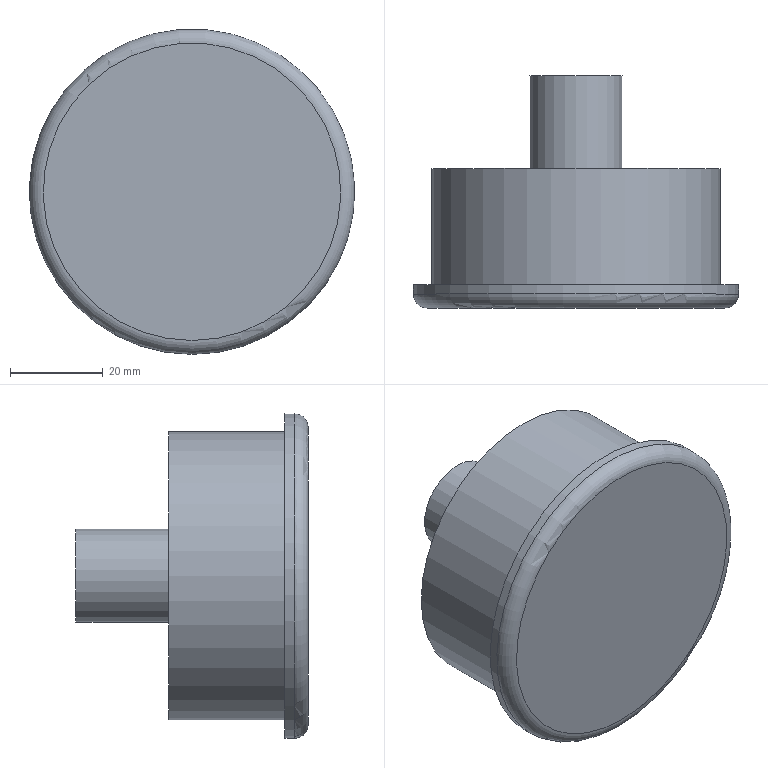Part | STEP file | Tube feed_id726_x_t | 1 solid | 8 faces | box 70 x 50 x 70 mm | volume 100586 mm3 | plane 4 | cylinder 3 | torus 1 | commonest cylinder face diameters 20 x1 62 x1 70 x1
STEP:
#1=CARTESIAN_POINT('',(0.,0.,0.));
#2=DIRECTION('',(0.,0.,1.));
#3=DIRECTION('',(1.,0.,0.));
#4=AXIS2_PLACEMENT_3D('',#1,#2,#3);
#5=CARTESIAN_POINT('',(581.,140.936,-4.));
#6=VERTEX_POINT('',#5);
#7=CARTESIAN_POINT('',(550.,140.936,-4.));
#8=DIRECTION('',(0.,-1.,0.));
#9=DIRECTION('',(1.,0.,0.));
#10=AXIS2_PLACEMENT_3D('',#7,#8,#9);
#11=CIRCLE('',#10,31.);
#12=CARTESIAN_POINT('',(550.,110.936,-4.));
#13=DIRECTION('',(0.,1.,0.));
#14=DIRECTION('',(0.,0.,1.));
#15=AXIS2_PLACEMENT_3D('',#12,#13,#14);
#16=CYLINDRICAL_SURFACE('',#15,31.);
#17=CARTESIAN_POINT('',(7.854,30.));
#18=DIRECTION('',(-1.,0.));
#19=VECTOR('',#18,1.);
#20=LINE('',#17,#19);
#21=(GEOMETRIC_REPRESENTATION_CONTEXT(2)PARAMETRIC_REPRESENTATION_CONTEXT()REPRESENTATION_CONTEXT('',''));
#22=DEFINITIONAL_REPRESENTATION('',(#20),#21);
#23=PCURVE('',#16,#22);
#24=CARTESIAN_POINT('',(550.,140.936,-4.));
#25=DIRECTION('',(0.,-1.,0.));
#26=DIRECTION('',(0.,0.,-1.));
#27=AXIS2_PLACEMENT_3D('',#24,#25,#26);
#28=PLANE('',#27);
#29=CARTESIAN_POINT('',(0.,0.));
#30=DIRECTION('',(0.,1.));
#31=AXIS2_PLACEMENT_2D('',#29,#30);
#32=CIRCLE('',#31,31.);
#33=(GEOMETRIC_REPRESENTATION_CONTEXT(2)PARAMETRIC_REPRESENTATION_CONTEXT()REPRESENTATION_CONTEXT('',''));
#34=DEFINITIONAL_REPRESENTATION('',(#32),#33);
#35=PCURVE('',#28,#34);
#36=SURFACE_CURVE('',#11,(#23,#35),.PCURVE_S1.);
#37=EDGE_CURVE('',#6,#6,#36,.T.);
#38=ORIENTED_EDGE('',*,*,#37,.T.);
#39=CARTESIAN_POINT('',(581.,115.936,-4.));
#40=VERTEX_POINT('',#39);
#41=CARTESIAN_POINT('',(581.,115.936,-4.));
#42=CARTESIAN_POINT('',(581.,140.936,-4.));
#43=B_SPLINE_CURVE_WITH_KNOTS('',1,(#41,#42),.UNSPECIFIED.,.F.,.F.,(2,2),(5.,30.),.PIECEWISE_BEZIER_KNOTS.);
#44=CARTESIAN_POINT('',(1.571,0.));
#45=DIRECTION('',(0.,1.));
#46=VECTOR('',#45,1.);
#47=LINE('',#44,#46);
#48=(GEOMETRIC_REPRESENTATION_CONTEXT(2)PARAMETRIC_REPRESENTATION_CONTEXT()REPRESENTATION_CONTEXT('',''));
#49=DEFINITIONAL_REPRESENTATION('',(#47),#48);
#50=PCURVE('',#16,#49);
#51=CARTESIAN_POINT('',(7.854,0.));
#52=DIRECTION('',(0.,1.));
#53=VECTOR('',#52,1.);
#54=LINE('',#51,#53);
#55=(GEOMETRIC_REPRESENTATION_CONTEXT(2)PARAMETRIC_REPRESENTATION_CONTEXT()REPRESENTATION_CONTEXT('',''));
#56=DEFINITIONAL_REPRESENTATION('',(#54),#55);
#57=PCURVE('',#16,#56);
#58=SEAM_CURVE('',#43,(#50,#57),.PCURVE_S1.);
#59=EDGE_CURVE('',#40,#6,#58,.T.);
#60=ORIENTED_EDGE('',*,*,#59,.F.);
#61=CARTESIAN_POINT('',(550.,115.936,-35.));
#62=VERTEX_POINT('',#61);
#63=CARTESIAN_POINT('',(550.,115.936,-4.));
#64=DIRECTION('',(0.,-1.,0.));
#65=DIRECTION('',(0.,0.,-1.));
#66=AXIS2_PLACEMENT_3D('',#63,#64,#65);
#67=CIRCLE('',#66,31.);
#68=CARTESIAN_POINT('',(3.142,5.));
#69=DIRECTION('',(-1.,0.));
#70=VECTOR('',#69,1.);
#71=LINE('',#68,#70);
#72=(GEOMETRIC_REPRESENTATION_CONTEXT(2)PARAMETRIC_REPRESENTATION_CONTEXT()REPRESENTATION_CONTEXT('',''));
#73=DEFINITIONAL_REPRESENTATION('',(#71),#72);
#74=PCURVE('',#16,#73);
#75=CARTESIAN_POINT('',(550.,115.936,-4.));
#76=DIRECTION('',(0.,-1.,0.));
#77=DIRECTION('',(0.,0.,-1.));
#78=AXIS2_PLACEMENT_3D('',#75,#76,#77);
#79=PLANE('',#78);
#80=CARTESIAN_POINT('',(0.,0.));
#81=DIRECTION('',(1.,0.));
#82=AXIS2_PLACEMENT_2D('',#80,#81);
#83=CIRCLE('',#82,31.);
#84=(GEOMETRIC_REPRESENTATION_CONTEXT(2)PARAMETRIC_REPRESENTATION_CONTEXT()REPRESENTATION_CONTEXT('',''));
#85=DEFINITIONAL_REPRESENTATION('',(#83),#84);
#86=PCURVE('',#79,#85);
#87=SURFACE_CURVE('',#67,(#74,#86),.PCURVE_S1.);
#88=EDGE_CURVE('',#62,#40,#87,.T.);
#89=ORIENTED_EDGE('',*,*,#88,.F.);
#90=CARTESIAN_POINT('',(550.,115.936,-4.));
#91=DIRECTION('',(0.,-1.,0.));
#92=DIRECTION('',(0.,0.,-1.));
#93=AXIS2_PLACEMENT_3D('',#90,#91,#92);
#94=CIRCLE('',#93,31.);
#95=CARTESIAN_POINT('',(9.425,5.));
#96=DIRECTION('',(-1.,0.));
#97=VECTOR('',#96,1.);
#98=LINE('',#95,#97);
#99=(GEOMETRIC_REPRESENTATION_CONTEXT(2)PARAMETRIC_REPRESENTATION_CONTEXT()REPRESENTATION_CONTEXT('',''));
#100=DEFINITIONAL_REPRESENTATION('',(#98),#99);
#101=PCURVE('',#16,#100);
#102=CARTESIAN_POINT('',(0.,0.));
#103=DIRECTION('',(1.,0.));
#104=AXIS2_PLACEMENT_2D('',#102,#103);
#105=CIRCLE('',#104,31.);
#106=(GEOMETRIC_REPRESENTATION_CONTEXT(2)PARAMETRIC_REPRESENTATION_CONTEXT()REPRESENTATION_CONTEXT('',''));
#107=DEFINITIONAL_REPRESENTATION('',(#105),#106);
#108=PCURVE('',#79,#107);
#109=SURFACE_CURVE('',#94,(#101,#108),.PCURVE_S1.);
#110=EDGE_CURVE('',#40,#62,#109,.T.);
#111=ORIENTED_EDGE('',*,*,#110,.F.);
#112=ORIENTED_EDGE('',*,*,#59,.T.);
#113=EDGE_LOOP('',(#38,#60,#89,#111,#112));
#114=FACE_BOUND('',#113,.T.);
#115=ADVANCED_FACE('',(#114),#16,.T.);
#116=CARTESIAN_POINT('',(550.,140.936,-14.));
#117=VERTEX_POINT('',#116);
#118=CARTESIAN_POINT('',(550.,140.936,-4.));
#119=DIRECTION('',(0.,-1.,0.));
#120=DIRECTION('',(0.,0.,-1.));
#121=AXIS2_PLACEMENT_3D('',#118,#119,#120);
#122=CIRCLE('',#121,10.);
#123=CARTESIAN_POINT('',(0.,0.));
#124=DIRECTION('',(1.,0.));
#125=AXIS2_PLACEMENT_2D('',#123,#124);
#126=CIRCLE('',#125,10.);
#127=(GEOMETRIC_REPRESENTATION_CONTEXT(2)PARAMETRIC_REPRESENTATION_CONTEXT()REPRESENTATION_CONTEXT('',''));
#128=DEFINITIONAL_REPRESENTATION('',(#126),#127);
#129=PCURVE('',#28,#128);
#130=CARTESIAN_POINT('',(550.,145.936,-4.));
#131=DIRECTION('',(0.,-1.,0.));
#132=DIRECTION('',(0.,0.,-1.));
#133=AXIS2_PLACEMENT_3D('',#130,#131,#132);
#134=CYLINDRICAL_SURFACE('',#133,10.);
#135=CARTESIAN_POINT('',(0.,5.));
#136=DIRECTION('',(1.,0.));
#137=VECTOR('',#136,1.);
#138=LINE('',#135,#137);
#139=(GEOMETRIC_REPRESENTATION_CONTEXT(2)PARAMETRIC_REPRESENTATION_CONTEXT()REPRESENTATION_CONTEXT('',''));
#140=DEFINITIONAL_REPRESENTATION('',(#138),#139);
#141=PCURVE('',#134,#140);
#142=SURFACE_CURVE('',#122,(#129,#141),.PCURVE_S1.);
#143=EDGE_CURVE('',#117,#117,#142,.T.);
#144=ORIENTED_EDGE('',*,*,#143,.T.);
#145=EDGE_LOOP('',(#144));
#146=FACE_BOUND('',#145,.T.);
#147=ORIENTED_EDGE('',*,*,#37,.F.);
#148=EDGE_LOOP('',(#147));
#149=FACE_BOUND('',#148,.T.);
#150=ADVANCED_FACE('',(#146,#149),#28,.F.);
#151=CARTESIAN_POINT('',(550.,113.936,-39.));
#152=VERTEX_POINT('',#151);
#153=CARTESIAN_POINT('',(550.,113.936,-4.));
#154=DIRECTION('',(0.,1.,0.));
#155=DIRECTION('',(0.,0.,-1.));
#156=AXIS2_PLACEMENT_3D('',#153,#154,#155);
#157=CIRCLE('',#156,35.);
#158=CARTESIAN_POINT('',(550.,115.936,-4.));
#159=DIRECTION('',(0.,-1.,0.));
#160=DIRECTION('',(0.,0.,-1.));
#161=AXIS2_PLACEMENT_3D('',#158,#159,#160);
#162=CYLINDRICAL_SURFACE('',#161,35.);
#163=CARTESIAN_POINT('',(6.283,2.));
#164=DIRECTION('',(-1.,0.));
#165=VECTOR('',#164,1.);
#166=LINE('',#163,#165);
#167=(GEOMETRIC_REPRESENTATION_CONTEXT(2)PARAMETRIC_REPRESENTATION_CONTEXT()REPRESENTATION_CONTEXT('',''));
#168=DEFINITIONAL_REPRESENTATION('',(#166),#167);
#169=PCURVE('',#162,#168);
#170=CARTESIAN_POINT('',(550.,113.936,-4.));
#171=DIRECTION('',(0.,-1.,0.));
#172=DIRECTION('',(0.,0.,-1.));
#173=AXIS2_PLACEMENT_3D('',#170,#171,#172);
#174=TOROIDAL_SURFACE('',#173,32.,3.);
#175=CARTESIAN_POINT('',(6.283,6.283));
#176=DIRECTION('',(-1.,0.));
#177=VECTOR('',#176,1.);
#178=LINE('',#175,#177);
#179=(GEOMETRIC_REPRESENTATION_CONTEXT(2)PARAMETRIC_REPRESENTATION_CONTEXT()REPRESENTATION_CONTEXT('',''));
#180=DEFINITIONAL_REPRESENTATION('',(#178),#179);
#181=PCURVE('',#174,#180);
#182=SURFACE_CURVE('',#157,(#169,#181),.PCURVE_S1.);
#183=EDGE_CURVE('',#152,#152,#182,.T.);
#184=ORIENTED_EDGE('',*,*,#183,.T.);
#185=CARTESIAN_POINT('',(550.,115.936,-39.));
#186=VERTEX_POINT('',#185);
#187=CARTESIAN_POINT('',(550.,115.936,-39.));
#188=CARTESIAN_POINT('',(550.,113.936,-39.));
#189=B_SPLINE_CURVE_WITH_KNOTS('',1,(#187,#188),.UNSPECIFIED.,.F.,.F.,(2,2),(0.,2.),.PIECEWISE_BEZIER_KNOTS.);
#190=CARTESIAN_POINT('',(0.,0.));
#191=DIRECTION('',(0.,1.));
#192=VECTOR('',#191,1.);
#193=LINE('',#190,#192);
#194=(GEOMETRIC_REPRESENTATION_CONTEXT(2)PARAMETRIC_REPRESENTATION_CONTEXT()REPRESENTATION_CONTEXT('',''));
#195=DEFINITIONAL_REPRESENTATION('',(#193),#194);
#196=PCURVE('',#162,#195);
#197=CARTESIAN_POINT('',(6.283,0.));
#198=DIRECTION('',(0.,1.));
#199=VECTOR('',#198,1.);
#200=LINE('',#197,#199);
#201=(GEOMETRIC_REPRESENTATION_CONTEXT(2)PARAMETRIC_REPRESENTATION_CONTEXT()REPRESENTATION_CONTEXT('',''));
#202=DEFINITIONAL_REPRESENTATION('',(#200),#201);
#203=PCURVE('',#162,#202);
#204=SEAM_CURVE('',#189,(#196,#203),.PCURVE_S1.);
#205=EDGE_CURVE('',#186,#152,#204,.T.);
#206=ORIENTED_EDGE('',*,*,#205,.F.);
#207=CARTESIAN_POINT('',(550.,115.936,-4.));
#208=DIRECTION('',(0.,-1.,0.));
#209=DIRECTION('',(0.,0.,-1.));
#210=AXIS2_PLACEMENT_3D('',#207,#208,#209);
#211=CIRCLE('',#210,35.);
#212=CARTESIAN_POINT('',(0.,0.));
#213=DIRECTION('',(1.,0.));
#214=VECTOR('',#213,1.);
#215=LINE('',#212,#214);
#216=(GEOMETRIC_REPRESENTATION_CONTEXT(2)PARAMETRIC_REPRESENTATION_CONTEXT()REPRESENTATION_CONTEXT('',''));
#217=DEFINITIONAL_REPRESENTATION('',(#215),#216);
#218=PCURVE('',#162,#217);
#219=CARTESIAN_POINT('',(0.,0.));
#220=DIRECTION('',(1.,0.));
#221=AXIS2_PLACEMENT_2D('',#219,#220);
#222=CIRCLE('',#221,35.);
#223=(GEOMETRIC_REPRESENTATION_CONTEXT(2)PARAMETRIC_REPRESENTATION_CONTEXT()REPRESENTATION_CONTEXT('',''));
#224=DEFINITIONAL_REPRESENTATION('',(#222),#223);
#225=PCURVE('',#79,#224);
#226=SURFACE_CURVE('',#211,(#218,#225),.PCURVE_S1.);
#227=EDGE_CURVE('',#186,#186,#226,.T.);
#228=ORIENTED_EDGE('',*,*,#227,.T.);
#229=ORIENTED_EDGE('',*,*,#205,.T.);
#230=EDGE_LOOP('',(#184,#206,#228,#229));
#231=FACE_BOUND('',#230,.T.);
#232=ADVANCED_FACE('',(#231),#162,.T.);
#233=ORIENTED_EDGE('',*,*,#88,.T.);
#234=ORIENTED_EDGE('',*,*,#110,.T.);
#235=EDGE_LOOP('',(#233,#234));
#236=FACE_BOUND('',#235,.T.);
#237=ORIENTED_EDGE('',*,*,#227,.F.);
#238=EDGE_LOOP('',(#237));
#239=FACE_BOUND('',#238,.T.);
#240=ADVANCED_FACE('',(#236,#239),#79,.F.);
#241=CARTESIAN_POINT('',(550.,110.936,-36.));
#242=VERTEX_POINT('',#241);
#243=CARTESIAN_POINT('',(550.,110.936,-4.));
#244=DIRECTION('',(0.,-1.,0.));
#245=DIRECTION('',(0.,0.,-1.));
#246=AXIS2_PLACEMENT_3D('',#243,#244,#245);
#247=CIRCLE('',#246,32.);
#248=CARTESIAN_POINT('',(550.,110.936,-4.));
#249=DIRECTION('',(0.,-1.,0.));
#250=DIRECTION('',(0.,0.,-1.));
#251=AXIS2_PLACEMENT_3D('',#248,#249,#250);
#252=PLANE('',#251);
#253=CARTESIAN_POINT('',(0.,0.));
#254=DIRECTION('',(1.,0.));
#255=AXIS2_PLACEMENT_2D('',#253,#254);
#256=CIRCLE('',#255,32.);
#257=(GEOMETRIC_REPRESENTATION_CONTEXT(2)PARAMETRIC_REPRESENTATION_CONTEXT()REPRESENTATION_CONTEXT('',''));
#258=DEFINITIONAL_REPRESENTATION('',(#256),#257);
#259=PCURVE('',#252,#258);
#260=CARTESIAN_POINT('',(0.,7.854));
#261=DIRECTION('',(1.,0.));
#262=VECTOR('',#261,1.);
#263=LINE('',#260,#262);
#264=(GEOMETRIC_REPRESENTATION_CONTEXT(2)PARAMETRIC_REPRESENTATION_CONTEXT()REPRESENTATION_CONTEXT('',''));
#265=DEFINITIONAL_REPRESENTATION('',(#263),#264);
#266=PCURVE('',#174,#265);
#267=SURFACE_CURVE('',#247,(#259,#266),.PCURVE_S1.);
#268=EDGE_CURVE('',#242,#242,#267,.T.);
#269=ORIENTED_EDGE('',*,*,#268,.T.);
#270=EDGE_LOOP('',(#269));
#271=FACE_BOUND('',#270,.T.);
#272=ADVANCED_FACE('',(#271),#252,.T.);
#273=ORIENTED_EDGE('',*,*,#183,.F.);
#274=CARTESIAN_POINT('',(550.,113.936,-39.));
#275=CARTESIAN_POINT('',(550.,113.134,-39.));
#276=CARTESIAN_POINT('',(550.,112.353,-38.745));
#277=CARTESIAN_POINT('',(550.,111.68,-38.256));
#278=CARTESIAN_POINT('',(550.,111.191,-37.583));
#279=CARTESIAN_POINT('',(550.,110.936,-36.802));
#280=CARTESIAN_POINT('',(550.,110.936,-36.));
#281=(BOUNDED_CURVE()B_SPLINE_CURVE(6,(#274,#275,#276,#277,#278,#279,#280),.UNSPECIFIED.,.F.,.F.)B_SPLINE_CURVE_WITH_KNOTS((7,7),(0.,1.571),.PIECEWISE_BEZIER_KNOTS.)CURVE()GEOMETRIC_REPRESENTATION_ITEM()RATIONAL_B_SPLINE_CURVE((1.031,1.01,0.9979,0.994,0.9979,1.01,1.031))REPRESENTATION_ITEM(''));
#282=CARTESIAN_POINT('',(6.283,6.283));
#283=DIRECTION('',(0.,1.));
#284=VECTOR('',#283,1.);
#285=LINE('',#282,#284);
#286=(GEOMETRIC_REPRESENTATION_CONTEXT(2)PARAMETRIC_REPRESENTATION_CONTEXT()REPRESENTATION_CONTEXT('',''));
#287=DEFINITIONAL_REPRESENTATION('',(#285),#286);
#288=PCURVE('',#174,#287);
#289=CARTESIAN_POINT('',(0.,6.283));
#290=DIRECTION('',(0.,1.));
#291=VECTOR('',#290,1.);
#292=LINE('',#289,#291);
#293=(GEOMETRIC_REPRESENTATION_CONTEXT(2)PARAMETRIC_REPRESENTATION_CONTEXT()REPRESENTATION_CONTEXT('',''));
#294=DEFINITIONAL_REPRESENTATION('',(#292),#293);
#295=PCURVE('',#174,#294);
#296=SEAM_CURVE('',#281,(#288,#295),.PCURVE_S1.);
#297=EDGE_CURVE('',#152,#242,#296,.T.);
#298=ORIENTED_EDGE('',*,*,#297,.T.);
#299=ORIENTED_EDGE('',*,*,#268,.F.);
#300=ORIENTED_EDGE('',*,*,#297,.F.);
#301=EDGE_LOOP('',(#273,#298,#299,#300));
#302=FACE_BOUND('',#301,.T.);
#303=ADVANCED_FACE('',(#302),#174,.T.);
#304=CARTESIAN_POINT('',(550.,160.936,6.));
#305=VERTEX_POINT('',#304);
#306=CARTESIAN_POINT('',(550.,160.936,-14.));
#307=VERTEX_POINT('',#306);
#308=CARTESIAN_POINT('',(550.,160.936,-4.));
#309=DIRECTION('',(0.,-1.,0.));
#310=DIRECTION('',(0.,0.,1.));
#311=AXIS2_PLACEMENT_3D('',#308,#309,#310);
#312=CIRCLE('',#311,10.);
#313=CARTESIAN_POINT('',(3.142,-15.));
#314=DIRECTION('',(1.,0.));
#315=VECTOR('',#314,1.);
#316=LINE('',#313,#315);
#317=(GEOMETRIC_REPRESENTATION_CONTEXT(2)PARAMETRIC_REPRESENTATION_CONTEXT()REPRESENTATION_CONTEXT('',''));
#318=DEFINITIONAL_REPRESENTATION('',(#316),#317);
#319=PCURVE('',#134,#318);
#320=CARTESIAN_POINT('',(536.,160.936,46.));
#321=DIRECTION('',(0.,1.,0.));
#322=DIRECTION('',(0.,0.,1.));
#323=AXIS2_PLACEMENT_3D('',#320,#321,#322);
#324=PLANE('',#323);
#325=CARTESIAN_POINT('',(-40.,14.));
#326=CARTESIAN_POINT('',(-40.,-3.321));
#327=CARTESIAN_POINT('',(-55.,5.34));
#328=CARTESIAN_POINT('',(-70.,14.));
#329=CARTESIAN_POINT('',(-55.,22.66));
#330=CARTESIAN_POINT('',(-40.,31.321));
#331=CARTESIAN_POINT('',(-40.,14.));
#332=(BOUNDED_CURVE()B_SPLINE_CURVE(2,(#325,#326,#327,#328,#329,#330,#331),.UNSPECIFIED.,.T.,.F.)B_SPLINE_CURVE_WITH_KNOTS((1,2,2,2,2,1),(-2.094,0.,2.094,4.189,6.283,8.378),.UNSPECIFIED.)CURVE()GEOMETRIC_REPRESENTATION_ITEM()RATIONAL_B_SPLINE_CURVE((1.,0.5,1.,0.5,1.,0.5,1.))REPRESENTATION_ITEM(''));
#333=(GEOMETRIC_REPRESENTATION_CONTEXT(2)PARAMETRIC_REPRESENTATION_CONTEXT()REPRESENTATION_CONTEXT('',''));
#334=DEFINITIONAL_REPRESENTATION('',(#332),#333);
#335=PCURVE('',#324,#334);
#336=SURFACE_CURVE('',#312,(#319,#335),.PCURVE_S1.);
#337=EDGE_CURVE('',#305,#307,#336,.T.);
#338=ORIENTED_EDGE('',*,*,#337,.T.);
#339=CARTESIAN_POINT('',(550.,160.936,-14.));
#340=CARTESIAN_POINT('',(550.,140.936,-14.));
#341=B_SPLINE_CURVE_WITH_KNOTS('',1,(#339,#340),.UNSPECIFIED.,.F.,.F.,(2,2),(-15.,5.),.PIECEWISE_BEZIER_KNOTS.);
#342=CARTESIAN_POINT('',(6.283,0.));
#343=DIRECTION('',(0.,1.));
#344=VECTOR('',#343,1.);
#345=LINE('',#342,#344);
#346=(GEOMETRIC_REPRESENTATION_CONTEXT(2)PARAMETRIC_REPRESENTATION_CONTEXT()REPRESENTATION_CONTEXT('',''));
#347=DEFINITIONAL_REPRESENTATION('',(#345),#346);
#348=PCURVE('',#134,#347);
#349=CARTESIAN_POINT('',(0.,0.));
#350=DIRECTION('',(0.,1.));
#351=VECTOR('',#350,1.);
#352=LINE('',#349,#351);
#353=(GEOMETRIC_REPRESENTATION_CONTEXT(2)PARAMETRIC_REPRESENTATION_CONTEXT()REPRESENTATION_CONTEXT('',''));
#354=DEFINITIONAL_REPRESENTATION('',(#352),#353);
#355=PCURVE('',#134,#354);
#356=SEAM_CURVE('',#341,(#348,#355),.PCURVE_S1.);
#357=EDGE_CURVE('',#307,#117,#356,.T.);
#358=ORIENTED_EDGE('',*,*,#357,.T.);
#359=ORIENTED_EDGE('',*,*,#143,.F.);
#360=ORIENTED_EDGE('',*,*,#357,.F.);
#361=CARTESIAN_POINT('',(550.,160.936,-4.));
#362=DIRECTION('',(0.,-1.,0.));
#363=DIRECTION('',(0.,0.,1.));
#364=AXIS2_PLACEMENT_3D('',#361,#362,#363);
#365=CIRCLE('',#364,10.);
#366=CARTESIAN_POINT('',(-3.142,-15.));
#367=DIRECTION('',(1.,0.));
#368=VECTOR('',#367,1.);
#369=LINE('',#366,#368);
#370=(GEOMETRIC_REPRESENTATION_CONTEXT(2)PARAMETRIC_REPRESENTATION_CONTEXT()REPRESENTATION_CONTEXT('',''));
#371=DEFINITIONAL_REPRESENTATION('',(#369),#370);
#372=PCURVE('',#134,#371);
#373=CARTESIAN_POINT('',(-40.,14.));
#374=CARTESIAN_POINT('',(-40.,-3.321));
#375=CARTESIAN_POINT('',(-55.,5.34));
#376=CARTESIAN_POINT('',(-70.,14.));
#377=CARTESIAN_POINT('',(-55.,22.66));
#378=CARTESIAN_POINT('',(-40.,31.321));
#379=CARTESIAN_POINT('',(-40.,14.));
#380=(BOUNDED_CURVE()B_SPLINE_CURVE(2,(#373,#374,#375,#376,#377,#378,#379),.UNSPECIFIED.,.T.,.F.)B_SPLINE_CURVE_WITH_KNOTS((1,2,2,2,2,1),(-2.094,0.,2.094,4.189,6.283,8.378),.UNSPECIFIED.)CURVE()GEOMETRIC_REPRESENTATION_ITEM()RATIONAL_B_SPLINE_CURVE((1.,0.5,1.,0.5,1.,0.5,1.))REPRESENTATION_ITEM(''));
#381=(GEOMETRIC_REPRESENTATION_CONTEXT(2)PARAMETRIC_REPRESENTATION_CONTEXT()REPRESENTATION_CONTEXT('',''));
#382=DEFINITIONAL_REPRESENTATION('',(#380),#381);
#383=PCURVE('',#324,#382);
#384=SURFACE_CURVE('',#365,(#372,#383),.PCURVE_S1.);
#385=EDGE_CURVE('',#307,#305,#384,.T.);
#386=ORIENTED_EDGE('',*,*,#385,.T.);
#387=EDGE_LOOP('',(#338,#358,#359,#360,#386));
#388=FACE_BOUND('',#387,.T.);
#389=ADVANCED_FACE('',(#388),#134,.T.);
#390=ORIENTED_EDGE('',*,*,#337,.F.);
#391=ORIENTED_EDGE('',*,*,#385,.F.);
#392=EDGE_LOOP('',(#390,#391));
#393=FACE_BOUND('',#392,.T.);
#394=ADVANCED_FACE('',(#393),#324,.T.);
#395=CLOSED_SHELL('',(#115,#150,#232,#240,#272,#303,#389,#394));
#396=MANIFOLD_SOLID_BREP('',#395);
#397=(LENGTH_UNIT()NAMED_UNIT(*)SI_UNIT(.MILLI.,.METRE.));
#398=UNCERTAINTY_MEASURE_WITH_UNIT(LENGTH_MEASURE(0.000005),#397,'','');
#399=(NAMED_UNIT(*)PLANE_ANGLE_UNIT()SI_UNIT($,.RADIAN.));
#400=(NAMED_UNIT(*)SI_UNIT($,.STERADIAN.)SOLID_ANGLE_UNIT());
#401=(GEOMETRIC_REPRESENTATION_CONTEXT(3)GLOBAL_UNCERTAINTY_ASSIGNED_CONTEXT((#398))GLOBAL_UNIT_ASSIGNED_CONTEXT((#397,#399,#400))REPRESENTATION_CONTEXT('',''));
#402=ADVANCED_BREP_SHAPE_REPRESENTATION('',(#4,#396),#401);